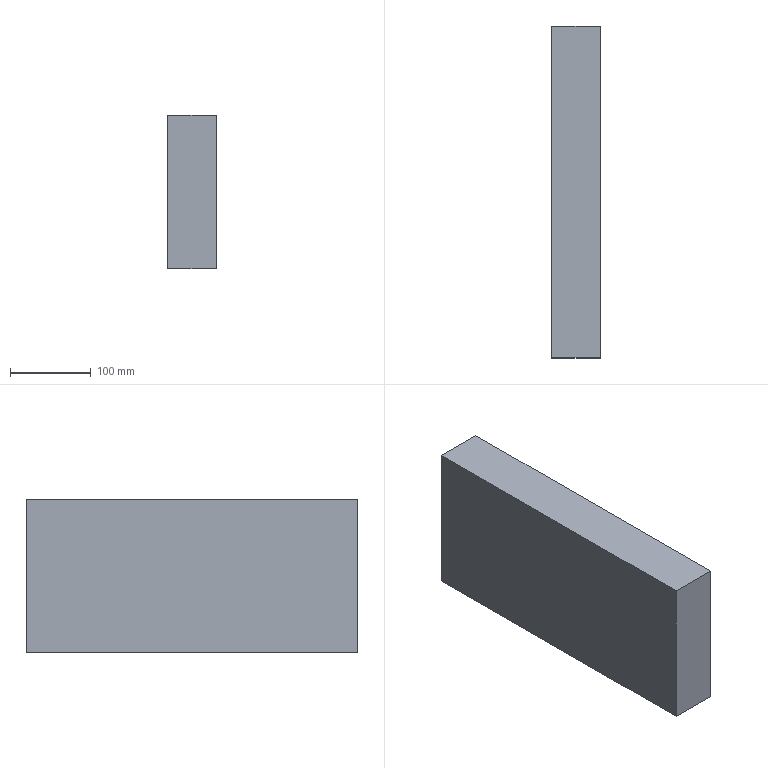Part | STEP file | lll_id4474_x_t | 1 solid | 10 faces | box 60 x 410 x 190 mm | volume 4652737 mm3 | plane 6 | cylinder 2 | cone 2 | commonest cylinder face diameters 17.506 x2
STEP:
#1=CARTESIAN_POINT('',(2331.188,165.,-370.));
#2=VERTEX_POINT('',#1);
#3=CARTESIAN_POINT('',(2322.435,165.,-370.));
#4=DIRECTION('',(0.,0.,1.));
#5=DIRECTION('',(1.,0.,0.));
#6=AXIS2_PLACEMENT_3D('',#3,#4,#5);
#7=CIRCLE('',#6,8.753);
#8=EDGE_CURVE('',#2,#2,#7,.T.);
#9=ORIENTED_EDGE('',*,*,#8,.T.);
#10=EDGE_LOOP('',(#9));
#11=FACE_BOUND('',#10,.T.);
#12=CARTESIAN_POINT('',(2352.435,205.,-370.));
#13=VERTEX_POINT('',#12);
#14=CARTESIAN_POINT('',(2352.435,-205.,-370.));
#15=VERTEX_POINT('',#14);
#16=CARTESIAN_POINT('',(2352.435,600.,-370.));
#17=DIRECTION('',(0.,-1.,0.));
#18=VECTOR('',#17,1.);
#19=LINE('',#16,#18);
#20=EDGE_CURVE('',#13,#15,#19,.T.);
#21=ORIENTED_EDGE('',*,*,#20,.T.);
#22=CARTESIAN_POINT('',(2292.435,-205.,-370.));
#23=VERTEX_POINT('',#22);
#24=CARTESIAN_POINT('',(4538.751,-205.,-370.));
#25=DIRECTION('',(-1.,0.,0.));
#26=VECTOR('',#25,1.);
#27=LINE('',#24,#26);
#28=EDGE_CURVE('',#15,#23,#27,.T.);
#29=ORIENTED_EDGE('',*,*,#28,.T.);
#30=CARTESIAN_POINT('',(2292.435,205.,-370.));
#31=VERTEX_POINT('',#30);
#32=CARTESIAN_POINT('',(2292.435,1.,-370.));
#33=DIRECTION('',(0.,-1.,0.));
#34=VECTOR('',#33,1.);
#35=LINE('',#32,#34);
#36=EDGE_CURVE('',#31,#23,#35,.T.);
#37=ORIENTED_EDGE('',*,*,#36,.F.);
#38=CARTESIAN_POINT('',(2322.435,205.,-370.));
#39=DIRECTION('',(-1.,0.,0.));
#40=VECTOR('',#39,1.);
#41=LINE('',#38,#40);
#42=EDGE_CURVE('',#13,#31,#41,.T.);
#43=ORIENTED_EDGE('',*,*,#42,.F.);
#44=EDGE_LOOP('',(#21,#29,#37,#43));
#45=FACE_BOUND('',#44,.T.);
#46=CARTESIAN_POINT('',(2331.188,-165.,-370.));
#47=VERTEX_POINT('',#46);
#48=CARTESIAN_POINT('',(2322.435,-165.,-370.));
#49=DIRECTION('',(0.,0.,1.));
#50=DIRECTION('',(1.,0.,0.));
#51=AXIS2_PLACEMENT_3D('',#48,#49,#50);
#52=CIRCLE('',#51,8.753);
#53=EDGE_CURVE('',#47,#47,#52,.T.);
#54=ORIENTED_EDGE('',*,*,#53,.T.);
#55=EDGE_LOOP('',(#54));
#56=FACE_BOUND('',#55,.T.);
#57=CARTESIAN_POINT('',(4538.751,1.,-370.));
#58=DIRECTION('',(0.,0.,-1.));
#59=DIRECTION('',(-1.,0.,0.));
#60=AXIS2_PLACEMENT_3D('',#57,#58,#59);
#61=PLANE('',#60);
#62=ADVANCED_FACE('',(#11,#45,#56),#61,.T.);
#63=CARTESIAN_POINT('',(2352.435,-205.,-180.));
#64=VERTEX_POINT('',#63);
#65=CARTESIAN_POINT('',(2352.435,-205.,-250.));
#66=DIRECTION('',(0.,0.,1.));
#67=VECTOR('',#66,1.);
#68=LINE('',#65,#67);
#69=EDGE_CURVE('',#15,#64,#68,.T.);
#70=ORIENTED_EDGE('',*,*,#69,.F.);
#71=ORIENTED_EDGE('',*,*,#20,.F.);
#72=CARTESIAN_POINT('',(2352.435,205.,-180.));
#73=VERTEX_POINT('',#72);
#74=CARTESIAN_POINT('',(2352.435,205.,-182.5));
#75=DIRECTION('',(0.,0.,1.));
#76=VECTOR('',#75,1.);
#77=LINE('',#74,#76);
#78=EDGE_CURVE('',#13,#73,#77,.T.);
#79=ORIENTED_EDGE('',*,*,#78,.T.);
#80=CARTESIAN_POINT('',(2352.435,1.,-180.));
#81=DIRECTION('',(0.,-1.,0.));
#82=VECTOR('',#81,1.);
#83=LINE('',#80,#82);
#84=EDGE_CURVE('',#73,#64,#83,.T.);
#85=ORIENTED_EDGE('',*,*,#84,.T.);
#86=EDGE_LOOP('',(#70,#71,#79,#85));
#87=FACE_OUTER_BOUND('',#86,.T.);
#88=CARTESIAN_POINT('',(2352.435,600.,-182.5));
#89=DIRECTION('',(1.,0.,0.));
#90=DIRECTION('',(0.,0.,-1.));
#91=AXIS2_PLACEMENT_3D('',#88,#89,#90);
#92=PLANE('',#91);
#93=ADVANCED_FACE('',(#87),#92,.T.);
#94=CARTESIAN_POINT('',(2292.435,205.,-180.));
#95=VERTEX_POINT('',#94);
#96=CARTESIAN_POINT('',(2322.435,205.,-180.));
#97=DIRECTION('',(-1.,0.,0.));
#98=VECTOR('',#97,1.);
#99=LINE('',#96,#98);
#100=EDGE_CURVE('',#73,#95,#99,.T.);
#101=ORIENTED_EDGE('',*,*,#100,.T.);
#102=CARTESIAN_POINT('',(2292.435,-205.,-180.));
#103=VERTEX_POINT('',#102);
#104=CARTESIAN_POINT('',(2292.435,0.,-180.));
#105=DIRECTION('',(0.,1.,0.));
#106=VECTOR('',#105,1.);
#107=LINE('',#104,#106);
#108=EDGE_CURVE('',#103,#95,#107,.T.);
#109=ORIENTED_EDGE('',*,*,#108,.F.);
#110=CARTESIAN_POINT('',(4538.751,-205.,-180.));
#111=DIRECTION('',(-1.,0.,0.));
#112=VECTOR('',#111,1.);
#113=LINE('',#110,#112);
#114=EDGE_CURVE('',#64,#103,#113,.T.);
#115=ORIENTED_EDGE('',*,*,#114,.F.);
#116=ORIENTED_EDGE('',*,*,#84,.F.);
#117=EDGE_LOOP('',(#101,#109,#115,#116));
#118=FACE_OUTER_BOUND('',#117,.T.);
#119=CARTESIAN_POINT('',(4538.751,1.,-180.));
#120=DIRECTION('',(0.,0.,-1.));
#121=DIRECTION('',(-1.,0.,0.));
#122=AXIS2_PLACEMENT_3D('',#119,#120,#121);
#123=PLANE('',#122);
#124=ADVANCED_FACE('',(#118),#123,.F.);
#125=CARTESIAN_POINT('',(2292.435,205.,-251.25));
#126=DIRECTION('',(0.,0.,1.));
#127=VECTOR('',#126,1.);
#128=LINE('',#125,#127);
#129=EDGE_CURVE('',#31,#95,#128,.T.);
#130=ORIENTED_EDGE('',*,*,#129,.F.);
#131=ORIENTED_EDGE('',*,*,#36,.T.);
#132=CARTESIAN_POINT('',(2292.435,-205.,-250.));
#133=DIRECTION('',(0.,0.,1.));
#134=VECTOR('',#133,1.);
#135=LINE('',#132,#134);
#136=EDGE_CURVE('',#23,#103,#135,.T.);
#137=ORIENTED_EDGE('',*,*,#136,.T.);
#138=ORIENTED_EDGE('',*,*,#108,.T.);
#139=EDGE_LOOP('',(#130,#131,#137,#138));
#140=FACE_OUTER_BOUND('',#139,.T.);
#141=CARTESIAN_POINT('',(2292.435,0.,-251.25));
#142=DIRECTION('',(1.,0.,0.));
#143=DIRECTION('',(0.,0.,-1.));
#144=AXIS2_PLACEMENT_3D('',#141,#142,#143);
#145=PLANE('',#144);
#146=ADVANCED_FACE('',(#140),#145,.F.);
#147=ORIENTED_EDGE('',*,*,#69,.T.);
#148=ORIENTED_EDGE('',*,*,#114,.T.);
#149=ORIENTED_EDGE('',*,*,#136,.F.);
#150=ORIENTED_EDGE('',*,*,#28,.F.);
#151=EDGE_LOOP('',(#147,#148,#149,#150));
#152=FACE_OUTER_BOUND('',#151,.T.);
#153=CARTESIAN_POINT('',(2322.435,-205.,-250.));
#154=DIRECTION('',(0.,-1.,0.));
#155=DIRECTION('',(0.,0.,-1.));
#156=AXIS2_PLACEMENT_3D('',#153,#154,#155);
#157=PLANE('',#156);
#158=ADVANCED_FACE('',(#152),#157,.T.);
#159=ORIENTED_EDGE('',*,*,#78,.F.);
#160=ORIENTED_EDGE('',*,*,#42,.T.);
#161=ORIENTED_EDGE('',*,*,#129,.T.);
#162=ORIENTED_EDGE('',*,*,#100,.F.);
#163=EDGE_LOOP('',(#159,#160,#161,#162));
#164=FACE_OUTER_BOUND('',#163,.T.);
#165=CARTESIAN_POINT('',(2322.435,205.,-250.));
#166=DIRECTION('',(0.,1.,0.));
#167=DIRECTION('',(0.,0.,1.));
#168=AXIS2_PLACEMENT_3D('',#165,#166,#167);
#169=PLANE('',#168);
#170=ADVANCED_FACE('',(#164),#169,.T.);
#171=CARTESIAN_POINT('',(2331.188,165.,-328.747));
#172=VERTEX_POINT('',#171);
#173=CARTESIAN_POINT('',(2322.435,165.,-328.747));
#174=DIRECTION('',(0.,0.,1.));
#175=DIRECTION('',(1.,0.,0.));
#176=AXIS2_PLACEMENT_3D('',#173,#174,#175);
#177=CIRCLE('',#176,8.753);
#178=EDGE_CURVE('',#172,#172,#177,.T.);
#179=ORIENTED_EDGE('',*,*,#178,.T.);
#180=EDGE_LOOP('',(#179));
#181=FACE_BOUND('',#180,.T.);
#182=ORIENTED_EDGE('',*,*,#8,.F.);
#183=EDGE_LOOP('',(#182));
#184=FACE_BOUND('',#183,.T.);
#185=CARTESIAN_POINT('',(2322.435,165.,-370.));
#186=DIRECTION('',(0.,0.,1.));
#187=DIRECTION('',(-1.,0.,0.));
#188=AXIS2_PLACEMENT_3D('',#185,#186,#187);
#189=CYLINDRICAL_SURFACE('',#188,8.753);
#190=ADVANCED_FACE('',(#181,#184),#189,.F.);
#191=CARTESIAN_POINT('',(2322.435,165.,-319.994));
#192=VERTEX_POINT('',#191);
#193=VERTEX_LOOP('',#192);
#194=FACE_BOUND('',#193,.T.);
#195=ORIENTED_EDGE('',*,*,#178,.F.);
#196=EDGE_LOOP('',(#195));
#197=FACE_BOUND('',#196,.T.);
#198=CARTESIAN_POINT('',(2322.435,165.,-328.747));
#199=DIRECTION('',(0.,0.,-1.));
#200=DIRECTION('',(1.,0.,0.));
#201=AXIS2_PLACEMENT_3D('',#198,#199,#200);
#202=CONICAL_SURFACE('',#201,8.753,45.);
#203=ADVANCED_FACE('',(#194,#197),#202,.F.);
#204=CARTESIAN_POINT('',(2331.188,-165.,-328.747));
#205=VERTEX_POINT('',#204);
#206=CARTESIAN_POINT('',(2322.435,-165.,-328.747));
#207=DIRECTION('',(0.,0.,1.));
#208=DIRECTION('',(1.,0.,0.));
#209=AXIS2_PLACEMENT_3D('',#206,#207,#208);
#210=CIRCLE('',#209,8.753);
#211=EDGE_CURVE('',#205,#205,#210,.T.);
#212=ORIENTED_EDGE('',*,*,#211,.T.);
#213=EDGE_LOOP('',(#212));
#214=FACE_BOUND('',#213,.T.);
#215=ORIENTED_EDGE('',*,*,#53,.F.);
#216=EDGE_LOOP('',(#215));
#217=FACE_BOUND('',#216,.T.);
#218=CARTESIAN_POINT('',(2322.435,-165.,-370.));
#219=DIRECTION('',(0.,0.,1.));
#220=DIRECTION('',(-1.,0.,0.));
#221=AXIS2_PLACEMENT_3D('',#218,#219,#220);
#222=CYLINDRICAL_SURFACE('',#221,8.753);
#223=ADVANCED_FACE('',(#214,#217),#222,.F.);
#224=CARTESIAN_POINT('',(2322.435,-165.,-319.994));
#225=VERTEX_POINT('',#224);
#226=VERTEX_LOOP('',#225);
#227=FACE_BOUND('',#226,.T.);
#228=ORIENTED_EDGE('',*,*,#211,.F.);
#229=EDGE_LOOP('',(#228));
#230=FACE_BOUND('',#229,.T.);
#231=CARTESIAN_POINT('',(2322.435,-165.,-328.747));
#232=DIRECTION('',(0.,0.,-1.));
#233=DIRECTION('',(1.,0.,0.));
#234=AXIS2_PLACEMENT_3D('',#231,#232,#233);
#235=CONICAL_SURFACE('',#234,8.753,45.);
#236=ADVANCED_FACE('',(#227,#230),#235,.F.);
#237=CLOSED_SHELL('',(#62,#93,#124,#146,#158,#170,#190,#203,#223,#236));
#238=MANIFOLD_SOLID_BREP('',#237);
#239=(LENGTH_UNIT()NAMED_UNIT(*)SI_UNIT(.MILLI.,.METRE.));
#240=UNCERTAINTY_MEASURE_WITH_UNIT(LENGTH_MEASURE(0.00002),#239,'','');
#241=(NAMED_UNIT(*)PLANE_ANGLE_UNIT()SI_UNIT($,.RADIAN.));
#242=PLANE_ANGLE_MEASURE_WITH_UNIT(PLANE_ANGLE_MEASURE(0.01745),#241);
#243=DIMENSIONAL_EXPONENTS(0.,0.,0.,0.,0.,0.,0.);
#244=(CONVERSION_BASED_UNIT('DEGREE',#242)NAMED_UNIT(#243)PLANE_ANGLE_UNIT());
#245=(NAMED_UNIT(*)SI_UNIT($,.STERADIAN.)SOLID_ANGLE_UNIT());
#246=(GEOMETRIC_REPRESENTATION_CONTEXT(3)GLOBAL_UNCERTAINTY_ASSIGNED_CONTEXT((#240))GLOBAL_UNIT_ASSIGNED_CONTEXT((#239,#244,#245))REPRESENTATION_CONTEXT('',''));
#247=ADVANCED_BREP_SHAPE_REPRESENTATION('',(#238),#246);